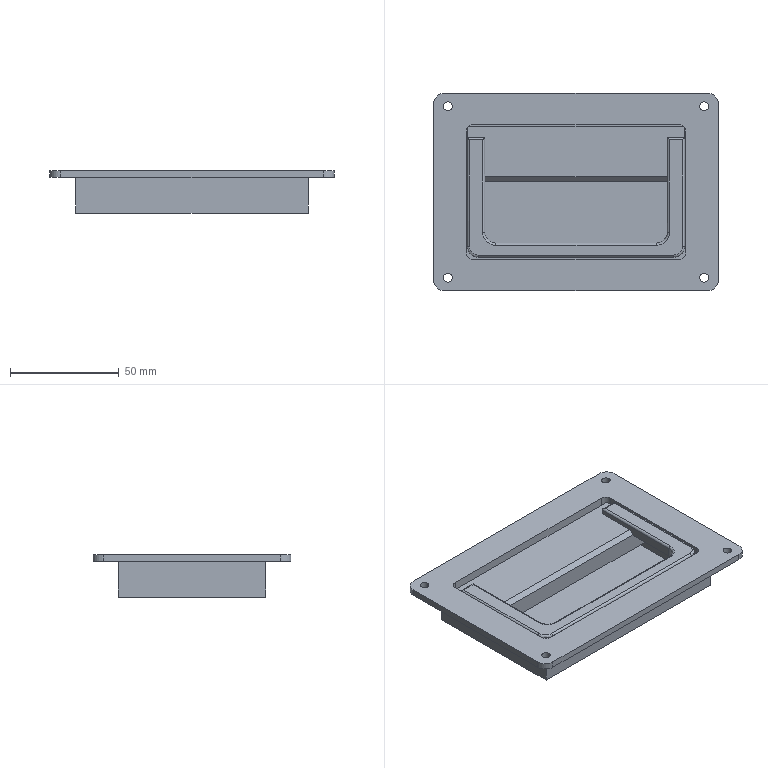Part | STEP file | HANDLE_130-91 | 1 solid | 63 faces | box 131 x 91 x 19.5 mm | volume 83642 mm3 | plane 31 | cylinder 28 | spline 4 | commonest cylinder face diameters 2 x8 4 x8 10 x8 6 x4